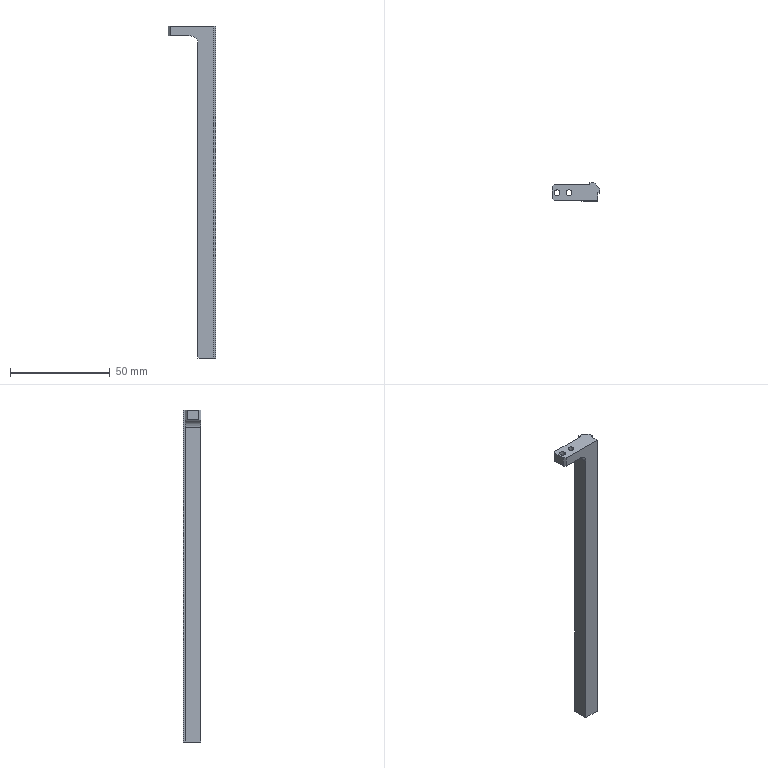NC program | NX | posted with a generic post | part box 24 x 9 x 166.5 mm
Whole program:
N10 G17 G21 G94 G90
(FACE_MILLING , TOOL : FACEMILL_D63)
N12 T01 M6
N14 G54
N16 G17 G0 G90 X-126.45 Y0. S4000 M3
N18 G43 Z20. H1
N20 G94 G1 Z0. F5000.
N22 X-117. F800.
N24 X117.
N26 X126.45
N28 G0 Z20.
N30 M5
(DYNAMIC_ROUGH , TOOL : D8-25-D8-60-3T-ROUGH)
N32 T02 M6
N34 G54
N36 G17 G0 G90 X92.04 Y3.501 S6500 M3
N38 G43 Z20. H2
N40 Z-10.5
N42 G94 G1 X92.015 Y3.499 Z-10.656 F3000.
N44 X91.991 Y3.497 Z-10.718
N46 X91.966 Y3.495 Z-10.763
N48 X91.941 Y3.493 Z-10.8
N50 X91.916 Y3.491 Z-10.831
N52 X91.891 Y3.489 Z-10.857
N54 X91.866 Y3.487 Z-10.88
N56 X91.841 Y3.485 Z-10.9
N58 X91.816 Y3.483 Z-10.918
N60 X91.791 Y3.481 Z-10.933
N62 X91.766 Y3.479 Z-10.947
N64 X91.741 Y3.477 Z-10.958
N66 X91.716 Y3.474 Z-10.968
N68 X91.692 Y3.472 Z-10.977
N70 X91.667 Y3.47 Z-10.984
N72 X91.642 Y3.468 Z-10.99
N74 X91.617 Y3.466 Z-10.994
N76 X91.592 Y3.464 Z-10.997
N78 X91.567 Y3.462 Z-10.999
N80 X91.542 Y3.46 Z-11.
N82 X90.193 Y3.35
N84 G3 X89.546 Y2.925 R0.809
N86 X88.822 Y0.359 R7.041
N88 X88.527 Y-5.709 R56.686
N90 G2 X88.481 Y-10.33 R413.5
N92 X86.629 Y-13.306 R4.525
N94 X82.787 Y-14.912 R9.339
N96 X77.117 Y-15.428 R33.802
N98 X65.718 Y-15.498 R574.286
N100 G1 X-75.866 Y-15.499
N102 G3 X-76.449 Y-15.739 R1.175
N104 G1 X-77.327 Y-16.046
N106 X-78.251 Y-16.15
N108 X-83.251
N110 X-84.173 Y-16.046
N112 X-85.051 Y-15.739
N114 X-85.837 Y-15.245
N116 X-86.495 Y-14.587
N118 G2 X-87.868 Y-11.251 R8.727
N120 X-88.416 Y-5.736 R30.867
N122 X-88.484 Y10.263 R613.548
N124 X-87.442 Y12.546 R4.163
N126 G3 X-87.296 Y12.923 R1.408
N128 G1 X-86.989 Y13.801
N130 X-86.495 Y14.587
N132 X-85.837 Y15.245
N134 X-85.051 Y15.739
N136 X-84.173 Y16.046
N138 X-83.249 Y16.15
N140 X83.251
N142 X84.173 Y16.046
N144 X85.051 Y15.739
N146 X85.837 Y15.245
N148 X86.495 Y14.587
N150 G2 X87.869 Y11.247 R8.729
N152 X88.36 Y4.982 R25.315
N154 G3 X87.818 Y-0.011 R824.39
N156 X87.514 Y-7.66 R117.924
N158 G2 X84.938 Y-12.045 R5.963
N160 X80.581 Y-13.828 R11.133
N162 X74.317 Y-14.417 R37.175
N164 X62.392 Y-14.497 R521.568
N166 G1 X-73.515 Y-14.498
N168 G3 X-74.911 Y-14.604 R5.765
N170 G1 X-75.177 Y-14.76
N172 G2 X-76.234 Y-15.604 R3.529
N174 G3 X-75.071 Y-14.653 R4.07
N176 G2 X-73.492 Y-14.176 R3.891
N178 X-68.214 Y-13.917 R44.777
N180 G1 X-61.946 Y-13.898
N182 X65.154 Y-13.896
N184 G3 X75.877 Y-13.729 R210.065
N186 X81.204 Y-12.923 R23.311
N188 X84.578 Y-11.011 R7.69
N190 X86.383 Y-7.437 R7.723
N192 X86.976 Y-3.056 R28.228
N194 G2 X87.641 Y4.04 R321.595
N196 G3 X87.4 Y9.877 R26.845
N198 G1 Y12.
N200 X87.296 Y12.923
N202 X86.989 Y13.801
N204 X87.296 Y12.923
N206 X87.4 Y12.
N208 Y2.999
N210 X87.296 Y2.077
N212 G3 X86.129 Y-2.669 R18.763
N214 G2 X85.377 Y-6.642 R25.565
N216 X81.646 Y-10.952 R7.379
N218 X76.555 Y-12.443 R15.205
N220 X68.997 Y-12.863 R64.21
N222 G1 X58.572 Y-12.897
N224 X-63.397 Y-12.898
N226 G3 X-71.446 Y-13.05 R128.548
N228 X-74.162 Y-13.532 R10.283
N230 X-74.52 Y-13.814 R1.243
N232 G2 X-75.111 Y-14.694 R4.84
N234 G3 X-74.476 Y-13.734 R4.989
N236 G2 X-73.386 Y-13.065 R2.302
N238 X-69.737 Y-12.458 R14.201
N240 X-61.269 Y-12.298 R147.584
N242 G1 X58.754
N244 G3 X71.903 Y-12.18 R390.996
N246 X78.003 Y-11.477 R31.973
N248 X82.054 Y-9.607 R9.974
N250 X84.616 Y-5.704 R8.61
N252 X85.652 Y-1.59 R35.363
N254 G2 X86.064 Y-0.063 R9.526
N256 X86.495 Y0.413 R2.986
N258 G1 X86.989 Y1.199
N260 X86.495 Y0.413
N262 G3 X85.019 Y-1.762 R5.148
N264 G2 X83.666 Y-5.178 R58.952
N266 X78.794 Y-9.678 R9.039
N268 X73.182 Y-10.954 R19.738
N270 X64.267 Y-11.281 R100.278
N272 G1 X55.417 Y-11.297
N274 X-60.696 Y-11.299
N276 G3 X-69.199 Y-11.472 R136.337
N278 X-73.009 Y-12.139 R14.86
N280 X-74.057 Y-12.703 R2.897
N282 G1 X-74.212 Y-12.945
N284 X-74.511 Y-13.801
N286 X-74.159 Y-12.781
N288 G2 X-72.878 Y-11.816 R2.774
N290 X-69.165 Y-10.98 R12.632
N292 X-61.331 Y-10.707 R88.006
N294 G1 X-56.096 Y-10.697
N296 X59.529 Y-10.695
N298 G3 X70.701 Y-10.513 R218.057
N300 X76.625 Y-9.641 R27.38
N302 X81.401 Y-6.811 R9.957
N304 X83.623 Y-3.265 R14.413
N306 G2 X84.842 Y-0.923 R20.753
N308 G1 X85.07 Y-0.727
N310 G3 X85.944 Y-0.139 R4.796
N312 G2 X84.781 Y-0.86 R4.613
N314 G3 X83.35 Y-2.41 R5.863
N316 G2 X81.221 Y-5.222 R26.449
N318 X75.576 Y-8.542 R12.045
N320 X69.359 Y-9.486 R29.39
N322 X58.412 Y-9.693 R196.812
N324 G1 X53.612 Y-9.697
N326 X-57.697 Y-9.698
N328 G3 X-67.413 Y-9.886 R158.154
N330 X-72.053 Y-10.679 R18.532
N332 X-73.935 Y-11.756 R4.815
N334 X-74.118 Y-12.156 R1.287
N336 G1 X-74.204 Y-12.923
N338 X-74.1 Y-12.001
N340 G2 X-73.215 Y-10.948 R2.12
N342 X-70.062 Y-9.741 R8.553
N344 X-64.019 Y-9.178 R36.636
N346 X-54.671 Y-9.097 R407.332
N348 G1 X56.754 Y-9.095
N350 G3 X68.152 Y-8.93 R254.128
N352 X74.536 Y-8.088 R32.345
N354 X81.433 Y-3.721 R12.634
N356 G2 X83.542 Y-1.329 R28.766
N358 X84.173 Y-1.046 R0.965
N360 G1 X84.952 Y-0.773
N362 G2 X84.029 Y-1.062 R4.368
N364 G3 X82.743 Y-1.58 R2.441
N366 X80.273 Y-3.64 R34.223
N368 G2 X72.75 Y-7.23 R16.232
N370 X65.522 Y-7.975 R43.439
N372 X52.623 Y-8.096 R414.666
N374 G1 X-54.025 Y-8.097
N376 G3 X-65.124 Y-8.251 R236.531
N378 X-70.762 Y-9.036 R26.178
N380 X-73.655 Y-10.5 R7.121
N382 X-74.1 Y-11.249 R1.158
N384 G1 Y-12.001
N386 Y-11.099
N388 G2 X-73.325 Y-9.95 R2.119
N390 X-70.262 Y-8.464 R7.844
N392 X-64.46 Y-7.665 R28.232
N394 X-53.62 Y-7.498 R223.232
N396 G1 X50.579 Y-7.497
N398 G3 X64.928 Y-7.382 R486.963
N400 X72.085 Y-6.672 R44.486
N402 X79.833 Y-3.063 R17.368
N404 G2 X82.394 Y-1.243 R19.765
N406 X83.249 Y-1.15 R1.904
N408 G1 X83.771 Y-1.091
N410 G2 X82.355 Y-1.15 R8.516
N412 G3 X80.216 Y-1.964 R6.073
N414 G2 X76.295 Y-4.076 R52.076
N416 X68.548 Y-6.048 R25.204
N418 X59.336 Y-6.467 R95.672
N420 G1 X48.011 Y-6.497
N422 X-53.423 Y-6.498
N424 G3 X-64.207 Y-6.685 R200.665
N426 X-70.135 Y-7.55 R28.08
N428 X-73.458 Y-9.212 R8.514
N430 X-74.067 Y-9.99 R1.925
N432 X-74.1 Y-11.143 R6.16
N434 G1 X-74.094 Y-9.943
N436 G2 X-73.045 Y-8.552 R2.913
N438 X-69.606 Y-6.946 R9.396
N440 X-63.581 Y-6.096 R30.323
N442 X-52.12 Y-5.898 R213.101
N444 G1 X48.404 Y-5.897
N446 G3 X63.203 Y-5.779 R503.536
N448 X71.032 Y-5.007 R48.745
N450 X77.985 Y-2.452 R24.546
N452 G2 X80.667 Y-1.172 R22.225
N454 X82.386 Y-1.15 R18.999
N456 G3 X79.868 Y-1.177 R32.283
N458 X77.171 Y-1.975 R13.915
N460 G2 X65.488 Y-4.599 R36.687
N462 X54.319 Y-4.887 R169.644
N464 G1 X46.819 Y-4.897
N466 X-51.848 Y-4.898
N468 G3 X-63.225 Y-5.108 R202.281
N470 X-69.609 Y-6.057 R30.448
N472 X-73.246 Y-7.838 R9.799
N474 X-74.053 Y-8.784 R2.728
N476 G1 X-74.1 Y-9.003
N478 Y-10.053
N480 Y-8.853
N482 G2 X-73.254 Y-7.517 R2.642
N484 X-69.927 Y-5.691 R8.827
N486 X-63.838 Y-4.602 R26.701
N488 X-53.984 Y-4.306 R133.89
N490 G1 X-49.346 Y-4.297
N492 X49.629 Y-4.295
N494 G3 X63.127 Y-4.118 R322.68
N496 X71.891 Y-2.989 R45.301
N498 X77.108 Y-1.356 R64.058
N500 G2 X77.842 Y-1.15 R18.45
N502 G1 X80.167
N504 G3 X76.25 Y-1.168 R168.279
N506 X72.386 Y-1.88 R38.541
N508 G2 X60.773 Y-3.172 R63.645
N510 X44.65 Y-3.297 R571.956
N512 G1 X-50.422 Y-3.298
N514 G3 X-62.248 Y-3.524 R206.989
N516 X-69.093 Y-4.54 R33.173
N518 X-73.034 Y-6.415 R11.137
N520 X-74.047 Y-7.547 R3.465
N522 G1 X-74.1 Y-7.783
N524 Y-8.908
N526 Y-7.633
N528 G2 X-73.177 Y-6.184 R2.873
N530 X-69.613 Y-4.223 R9.627
N532 X-63.151 Y-3.036 R28.232
N534 X-53.003 Y-2.71 R131.453
N536 G1 X-45.221 Y-2.697
N538 X47.754 Y-2.695
N540 G3 X61.702 Y-2.522 R360.141
N542 X72.889 Y-1.15 R67.055
N544 G1 X76.564
N546 G3 X67.491 Y-1.167 R617.669
N548 G2 X50.94 Y-1.685 R225.211
N550 G1 X38.49 Y-1.697
N552 X-47.874 Y-1.699
N554 G3 X-60.624 Y-1.898 R264.925
N556 X-68.101 Y-2.877 R39.862
N558 X-72.564 Y-4.769 R13.517
N560 X-74.011 Y-6.2 R5.343
N562 G1 X-74.1 Y-6.525
N564 Y-7.65
N566 Y-6.375
N568 G2 X-73.239 Y-4.951 R2.853
N570 X-69.73 Y-2.886 R9.624
N572 X-63.172 Y-1.533 R27.214
N574 X-55.321 Y-1.15 R96.17
N576 G1 X67.829
N578 X67.964 Y-1.163
N580 X68.096 Y-1.195
N582 X69.068 Y-1.535
N584 G2 X68.802 Y-3.106 R0.808
N586 G1 X68.777 Z-10.999
N588 X68.752 Z-10.997
N590 X68.727 Z-10.994
N592 X68.702 Z-10.99
N594 X68.677 Z-10.984
N596 X68.652 Z-10.977
N598 X68.627 Z-10.968
N600 X68.602 Z-10.958
N602 X68.577 Z-10.947
N604 X68.552 Z-10.933
N606 X68.527 Z-10.918
N608 X68.502 Z-10.9
N610 X68.477 Z-10.88
N612 X68.452 Z-10.857
N614 X68.427 Z-10.831
N616 X68.402 Z-10.8
N618 X68.377 Z-10.763
N620 X68.352 Z-10.718
N622 X68.327 Z-10.656
N624 X68.302 Z-10.5
N626 G0 Z20.
N628 X-53.07
N630 Z-10.5
N632 G1 X-53.095 Z-10.656
N634 X-53.12 Z-10.718
N636 X-53.145 Z-10.763
N638 X-53.17 Z-10.8
N640 X-53.195 Z-10.831
N642 X-53.22 Z-10.857
N644 X-53.245 Z-10.88
N646 X-53.27 Z-10.9
N648 X-53.295 Z-10.918
N650 X-53.32 Z-10.933
N652 X-53.345 Z-10.947
N654 X-53.37 Z-10.958
N656 X-53.395 Z-10.968
N658 X-53.42 Z-10.977
N660 X-53.445 Z-10.984
N662 X-53.47 Z-10.99
N664 X-53.495 Z-10.994
N666 X-53.52 Z-10.997
N668 X-53.545 Z-10.999
N670 X-53.57 Z-11.
N672 G2 X-54.354 Y-2.493 R0.808
N674 G1 X-54.537 Y-1.762
N676 G3 X-55.321 Y-1.15 R0.808
N678 G1 X-65.683 Y-1.165
N680 G3 X-72.089 Y-3.135 R14.586
N682 X-73.992 Y-4.866 R6.277
N684 X-74.1 Y-5.224 R2.837
N686 G1 Y-6.424
N688 Y-5.074
N690 G2 X-73.187 Y-3.589 R3.012
N692 X-69.564 Y-1.491 R9.657
N694 X-68.387 Y-1.15 R13.019
N696 G1 X-65.387
N698 X-69.641 Y-1.16
N700 G3 X-73.974 Y-3.582 R6.322
N702 X-74.1 Y-3.977 R1.533
N704 G1 Y-5.102
N706 Y-3.827
N708 G2 X-73.161 Y-2.356 R2.822
N710 X-71.126 Y-1.157 R5.202
N712 G1 X-69.488 Y-1.15
N714 X-71.724 Y-1.165
N716 G3 X-74.016 Y-2.611 R3.408
N718 G1 X-74.1 Y-2.924
N720 Y-3.899
N722 Y-2.774
N724 G2 X-73.156 Y-1.486 R2.195
N726 X-72.429 Y-1.15 R1.55
N728 G1 X-71.529
N730 G3 X-72.871 Y-1.169 R29.249
N732 X-74.008 Y-1.912 R1.692
N734 G1 X-74.1 Y-2.245
N736 Y-2.845
N738 X-74.093 Y-2.02
N740 G2 X-73.128 Y-1.15 R1.19
N742 G1 X-72.678
N744 X-73.429 Y-1.172
N746 G3 X-74.1 Y-2.162 R0.89
N748 X-73.737 Y-2.833 R0.801
N750 G1 X-73.458 Y-3.014
N752 X-72.147 Y-3.869 Z-10.9
N754 G2 X-71.78 Y-4.16 R1.373 F15000.
N756 X-71.611 Y-4.652 R0.808
N758 G1 Y-11.986
N760 G2 X-72.155 Y-14.815 R7.625
N762 G1 X-72.298 Y-15.169
N764 X-72.449 Y-15.52
N766 G2 X-73.493 Y-16.742 R3.323
N768 X-75.768 Y-18.159 R22.76
N770 X-77.409 Y-18.578 R4.415
N772 G1 X-83.488 Y-18.972
N774 G2 X-85.925 Y-18.191 R3.495
N776 G1 X-86.989 Y-17.321
N778 G2 X-87.275 Y-16.592 R0.801
N780 G1 X-87.068 Y-15.042 Z-11. F3000.
N782 X-86.951 Y-14.171
N784 G3 X-86.989 Y-13.801 R0.843
N786 G1 X-87.296 Y-12.923
N788 X-87.4 Y-11.999
N790 Y12.001
N792 X-87.299 Y12.895
N794 G3 X-87.714 Y13.694 R0.809
N796 G1 X-88.876 Y14.331
N798 X-88.898 Y14.343 Z-10.999
N800 X-88.92 Y14.355 Z-10.997
N802 X-88.941 Y14.367 Z-10.994
N804 X-88.963 Y14.379 Z-10.99
N806 X-88.985 Y14.391 Z-10.984
N808 X-89.007 Y14.403 Z-10.977
N810 X-89.029 Y14.415 Z-10.968
N812 X-89.051 Y14.427 Z-10.958
N814 X-89.073 Y14.439 Z-10.947
N816 X-89.095 Y14.451 Z-10.933
N818 X-89.117 Y14.463 Z-10.918
N820 X-89.139 Y14.475 Z-10.9
N822 X-89.161 Y14.487 Z-10.88
N824 X-89.183 Y14.499 Z-10.857
N826 X-89.205 Y14.511 Z-10.831
N828 X-89.227 Y14.523 Z-10.8
N830 X-89.248 Y14.535 Z-10.763
N832 X-89.27 Y14.547 Z-10.718
N834 X-89.292 Y14.559 Z-10.656
N836 X-89.314 Y14.571 Z-10.5
N838 G0 Z20.
N840 M5
(PLANAR_MILL_COPY_1_COPY_COPY , TOOL : D8R0-FINISH)
N842 T03 M6
N844 G54
N846 G17 G0 G90 X88.25 Y4. S6500 M3
N848 G43 Z20. H3
N850 G94 G1 Z-11. F5000.
N852 G3 X87.25 Y3. R1. F500.
N854 G2 X83.25 Y-1. R4.
N856 G1 X-65.45
N858 X-74.25 F250.
N860 G2 X-74.15 Y-1.889 R4.
N862 G1 Y-5.393
N864 Y-12. F500.
N866 G2 X-78.15 Y-16. R4.
N868 G1 X-83.25
N870 G2 X-87.25 Y-12. R4.
N872 G1 Y12.
N874 G2 X-83.25 Y16. R4.
N876 G1 X83.25
N878 G2 X87.25 Y12. R4.
N880 G1 Y3.
N882 G3 X88.25 Y2. R1.
N884 G1 Y4.
N886 G3 X87.25 Y3. R1.
N888 G2 X83.25 Y-1. R4.
N890 G1 X-65.45
N892 X-74.25 F250.
N894 G2 X-74.15 Y-1.889 R4.
N896 G1 Y-5.393
N898 Y-12. F500.
N900 G2 X-78.15 Y-16. R4.
N902 G1 X-83.25
N904 G2 X-87.25 Y-12. R4.
N906 G1 Y12.
N908 G2 X-83.25 Y16. R4.
N910 G1 X83.25
N912 G2 X87.25 Y12. R4.
N914 G1 Y3.
N916 G3 X88.25 Y2. R1.
N918 G0 Z20.
N920 M5
(PLANAR_MILL_2 , TOOL : DJ-D3)
N922 T08 M6
N924 G54
N926 G17 G0 G90 X87.063 Y1.826 S3500 M3
N928 G43 Z20. H8
N930 Z1.
N932 G94 G1 Z-1. F1000.
N934 G41 X86.078 Y2. D8
N936 X83.249
N938 X-74.25
N940 G3 X-77.175 Y-1.667 R3.
N942 G2 X-77.15 Y-1.889 R1.
N944 G1 Y-12.
N946 G2 X-78.15 Y-13. R1.
N948 G1 X-83.25
N950 G2 X-84.25 Y-12. R1.
N952 G1 Y12.
N954 G2 X-83.25 Y13. R1.
N956 G1 X83.25
N958 G2 X84.25 Y12. R1.
N960 G1 Y3.001
N962 Y0.172
N964 G40
N966 X84.424 Y-0.813
N968 Z1.
N970 G0 Z20.
(PLANAR_MILL_2_COPY , TOOL : DJ-D3)
N972 X-74.065 Y-12.474
N974 Z0.8
N976 G1 Z-1.2 F600.
N978 G41 X-75.05 Y-12.3
N980 X-78.25
N982 X-83.25
N984 X-86.45
N986 G40
N988 X-87.435 Y-12.474
N990 Z0.8
N992 G0 Z20.
(PLANAR_MILL_2_COPY_COPY , TOOL : DJ-D3)
N994 X-74.065 Y-12.374
N996 Z0.8
N998 G1 Z-1.2
N1000 G41 X-75.05 Y-12.2
N1002 X-78.25
N1004 X-83.25
N1006 X-86.45
N1008 G40
N1010 X-87.435 Y-12.374
N1012 Z0.8
N1014 G0 Z20.
N1016 M5
(DRILLING_2 , TOOL : DJ-D8)
N1018 T04 M6
N1020 G54
N1022 G17 G0 G90 X-8.5 Y4. S2000 M3
N1024 G43 Z20. H4
N1026 G94 G81 G99 Z-1.5 F200. R3.
N1028 X-2.5
N1030 G80
N1032 G0 X-2.5 Y4. Z20.
N1034 M5
(DRILLING_2_COPY , TOOL : DRILL_D2.9-39-67)
N1036 T08 M6
N1038 G54
N1040 G17 G0 G90 X-8.5 Y4. S2500 M3
N1042 G43 Z20. H8
N1044 G94 G81 G99 Z-7. F200. R3.
N1046 X-2.5
N1048 G80
N1050 G0 X-2.5 Y4. Z20.
N1052 M5
(DRILLING_3 , TOOL : DJ-D3)
N1054 M6
N1056 G54
N1058 G17 G0 G90 X-5.03 Y-2.97 S2000 M3
N1060 G43 Z20. H8
N1062 G94 G81 G99 Z-1. F200. R3.
N1064 X-1.84 Y-6.16
N1066 G80
N1068 G0 X-1.84 Y-6.16 Z20.
N1070 M5
(DRILLING_3_COPY , TOOL : D1.8_DRILL)
N1072 T06 M6
N1074 G54
N1076 G17 G0 G90 X-1.84 Y-6.16 S2000 M3
N1078 G43 Z20. H6
N1080 G94 G83 G99 Z-8. F200. Q1.5 R3.
N1082 X-5.03 Y-2.97
N1084 G80
N1086 G0 X-5.03 Y-2.97 Z20.
N1088 M5
(FACE_MILLING_COPY , TOOL : D50)
N1090 T01 M6
N1092 G54
N1094 G17 G0 G90 X0. Y115.75 S4000 M3
N1096 G43 Z26. H1
N1098 G94 G1 Z5.025 F5000.
N1100 Y108.25 F1500.
N1102 Y-108.25
N1104 Y-115.75
N1106 G0 Z16.
N1108 Y115.75
N1110 G1 Z4.05 F5000.
N1112 Y108.25 F1500.
N1114 Y-108.25
N1116 Y-115.75
N1118 G0 Z16.
N1120 Y115.75
N1122 G1 Z3.075 F5000.
N1124 Y108.25 F1500.
N1126 Y-108.25
N1128 Y-115.75
N1130 G0 Z16.
N1132 Y115.75
N1134 G1 Z2.1 F5000.
N1136 Y108.25 F1500.
N1138 Y-108.25
N1140 Y-115.75
N1142 G0 Z16.
N1144 Y115.75
N1146 G1 Z1.125 F5000.
N1148 Y108.25 F1500.
N1150 Y-108.25
N1152 Y-115.75
N1154 G0 Z16.
N1156 Y115.75
N1158 G1 Z0.15 F5000.
N1160 Y108.25 F1500.
N1162 Y-108.25
N1164 Y-115.75
N1166 G0 Z26.
(FACE_MILLING_COPY_COPY , TOOL : D50)
N1168 Y115.75
N1170 G1 Z0. F5000.
N1172 Y108.25 F800.
N1174 Y-108.25
N1176 Y-115.75
N1178 G0 Z26.
(PLANAR_MILL , TOOL : D50)
N1180 X18.5 Y133.25
N1182 Z20.
N1184 Z2.1
N1186 G1 Z-0.9 F600.
N1188 Y83.25
N1190 Y-83.25
N1192 Y-133.25
N1194 Z2.1
N1196 G0 Z20.
N1198 M5
(PLANAR_MILL_COPY_2 , TOOL : D8-25-D8-60-3T-FINISH)
N1200 T03 M6
N1202 G54
N1204 G17 G0 G90 X-0.6 Y72.25 S5500 M3
N1206 G43 Z19. H3
N1208 G94 G1 Z-1. F5000.
N1210 Y78.25 F1500.
N1212 Y83.25
N1214 Y89.25
N1216 G0 Z4.
N1218 X4.2 Y72.25
N1220 G1 Z-1. F5000.
N1222 Y78.25 F1500.
N1224 Y83.25
N1226 Y89.25
N1228 G0 Z4.
N1230 X9. Y72.25
N1232 G1 Z-1. F5000.
N1234 Y78.25 F1500.
N1236 Y83.25
N1238 Y89.25
N1240 G0 Z19.
(PLANAR_MILL_COPY_2_COPY , TOOL : D8-25-D8-60-3T-FINISH)
N1242 Z20.
N1244 X-2.9 Y89.25
N1246 G1 Z-0.9 F5000.
N1248 Y83.25 F1500.
N1250 Y-83.25
N1252 Y-89.25
N1254 G0 Z20.
(PLANAR_MILL_COPY_2_COPY_COPY , TOOL : D8-25-D8-60-3T-FINISH)
N1256 X-3. Y89.25
N1258 G1 Z-1. F5000.
N1260 Y83.25 F800.
N1262 Y-83.25
N1264 Y-89.25
N1266 G0 Z20.
N1268 M5
(DRILLING , TOOL : DJ-D3)
N1270 T04 M6
N1272 G54
N1274 G17 G0 G90 X-4.5 Y24. S2000 M3
N1276 G43 Z29. H4
N1278 G94 G81 G99 Z-2.1 F200. R0.
N1280 G0 Z29.
N1282 G81 Y-36. Z-2.1 R0.
N1284 G0 Z29.
N1286 G80
N1288 G0 X-4.5 Y-36. Z29.
(PLANAR_MILL_COPY_2_COPY_1_COPY_1 , TOOL : DJ-D3)
N1290 X-14.75 Y83.15 S5000
N1292 Z20.
N1294 G1 Z-0.6 F5000.
N1296 G41 X-12.5 F1000. D4
N1298 G2 X-11.9 Y83.75 R0.6
N1300 G1 X-7.1
N1302 G2 X-6.5 Y83.15 R0.6
N1304 G1 Y-83.15
N1306 G2 X-7.1 Y-83.75 R0.6
N1308 G1 X-11.9
N1310 G2 X-12.5 Y-83.15 R0.6
N1312 G1 Y83.15
N1314 G40
N1316 X-14.75
N1318 G0 Z20.
(PLANAR_MILL_COPY_2_COPY_1_COPY_1_COPY , TOOL : DJ-D3)
N1320 X-5.997 Y85.35
N1322 Z19.
N1324 G1 Z0. F5000.
N1326 Z-2. F1000.
N1328 G41 X-6. Y85.15
N1330 G3 X-5. Y84.15 R1.
N1332 G1 X11.9
N1334 G2 X12.9 Y83.15 R1.
N1336 G1 Y78.35
N1338 G2 X11.9 Y77.35 R1.
N1340 G1 X11.336
N1342 G2 X10.9 Y77.25 R1.
N1344 G1 X0.219
N1346 G3 X-2.1 Y74.25 R3.1
N1348 G1 Y-83.25
N1350 Y-84.75
N1352 G40
N1354 X-2.097 Y-84.95
N1356 G0 Z19.
(PLANAR_MILL_COPY_2_COPY_1_COPY_1_COPY_COPY , TOOL : DJ-D3)
N1358 X12.303 Y85.65
N1360 G1 Z-0.2 F5000.
N1362 Z-2.2 F600.
N1364 G41 X12.3 Y83.25
N1366 Y78.25
N1368 Y76.05
N1370 G40
N1372 X12.303 Y75.85
N1374 Z-0.2
N1376 G0 Z19.
(PLANAR_MILL_COPY_2_COPY_1_COPY_1_COPY_COPY_COPY , TOOL : DJ-D3)
N1378 X12.203 Y85.65
N1380 G1 Z-0.2 F5000.
N1382 Z-2.2 F600.
N1384 G41 X12.2 Y83.25
N1386 Y78.25
N1388 Y76.05
N1390 G40
N1392 X12.203 Y75.85
N1394 Z-0.2
N1396 G0 Z19.
N1398 M5
(DRILLING_COPY , TOOL : D1.8_DRILL)
N1400 T06 M6
N1402 G54
N1404 G17 G0 G90 X-4.5 Y24. S2000 M3
N1406 G43 Z29. H6
N1408 G94 G81 G99 Z-7.5 F100. R0.
N1410 G0 Z29.
N1412 G81 Y-36. Z-7.5 R0.
N1414 G0 Z29.
N1416 G80
N1418 G0 X-4.5 Y-36. Z29.
N1420 M5
(PLANAR_MILL_3 , TOOL : DJ-D3)
N1422 T00 M6
N1424 G54
N1426 G17 G0 G90 X-8.3 Y-7.8 S4500 M3
N1428 G43 Z20. H0
N1430 Z1.7
N1432 G94 G1 Z-1.3 F800.
N1434 Y-5.
N1436 Y0.
N1438 Y2.8
N1440 Z1.7
N1442 G0 Z20.
N1444 X0.3
N1446 Z1.7
N1448 G1 Z-1.3
N1450 Y0.
N1452 Y-5.
N1454 Y-7.8
N1456 Z1.7
N1458 G0 Z20.
(DRILLING_1 , TOOL : DJ-D3)
N1460 X-1.5 Y-115.25 S2500
N1462 G81 G99 Z-16.1 F200. R-12.
N1464 G80
N1466 G0 X-1.5 Y-115.25 Z20.
N1468 M5
(DRILLING_1_COPY , TOOL : DRILL_D2.3-29-55)
N1470 M6
N1472 G54
N1474 G17 G0 G90 X-1.5 Y-115.25 S2500 M3
N1476 G43 Z20. H0
N1478 G94 G81 G99 Z-22. F200. R-12.
N1480 G80
N1482 G0 X-1.5 Y-115.25 Z20.
N1484 M5
(DRILLING_1_COPY_COPY , TOOL : FORMTAP_M2.5-12-D3-39)
N1486 M6
N1488 G54
N1490 G17 G0 G90 X-1.5 Y-115.25 S300 M3
N1492 G43 Z20. H0
N1494 G84 G94 G99 Z-21. F135. R-12.
N1496 G80
N1498 G0 X-1.5 Y-115.25 Z20.
N1500 M5
(PLANAR_MILL_COPY_2_COPY_1_COPY_1_COPY_1 , TOOL : D8-25-D8-60-3T-ROUGH)
N1502 T02 M6
N1504 G54
N1506 G17 G0 G90 X-0.1 Y-172.5 S5000 M3
N1508 G43 Z21. H2
N1510 G94 G1 Z0.1 F5000.
N1512 Y-166.5 F1200.
N1514 Y0.
N1516 Y6.
N1518 G0 Z21.
(ZLEVEL_PROFILE , TOOL : D8-25-D8-60-3T-ROUGH)
N1520 X10.712 Y5.2
N1522 G1 Z0.5 F5000.
N1524 Y0. F3000.
N1526 Y-166.5
N1528 Y-171.7
N1530 G0 X11.212 Z0.
N1532 G1 Y-166.5
N1534 Y0.
N1536 Y5.2
N1538 G0 X11.712 Z-0.5
N1540 G1 Y0.
N1542 Y-166.5
N1544 Y-171.7
N1546 G0 X12.212 Z-1.
N1548 G1 Y-166.5
N1550 Y0.
N1552 Y5.2
N1554 G0 X12.712 Z-1.5
N1556 G1 Y0.
N1558 Y-166.5
N1560 Y-171.7
N1562 G0 Z21.
N1564 M5
(PLANAR_MILL_COPY_2_COPY_1_COPY_1_COPY_1_COPY_2 , TOOL : D8R0-FINISH)
N1566 T03 M6
N1568 G54
N1570 G17 G0 G90 X0. Y-172.5 S5000 M3
N1572 G43 Z21. H3
N1574 G94 G1 Z0. F5000.
N1576 Y-166.5 F1200.
N1578 Y0.
N1580 Y6.
N1582 G0 Z21.
N1584 M5
(PLANAR_MILL_COPY_2_COPY_1_COPY_1_COPY_1_COPY_COPY , TOOL : DJ-D8)
N1586 T08 M6
N1588 G54
N1590 G17 G0 G90 X9.509 Y6.5 S5000 M3
N1592 G43 Z21. H8
N1594 G94 G1 Z-2.5 F5000.
N1596 G41 X9.5 Y6. F800. D8
N1598 Y0.
N1600 Y-166.5
N1602 Y-172.5
N1604 G40
N1606 X9.509 Y-173.
N1608 G0 Z21.
N1610 M5
(DRILLING_COPY_1 , TOOL : DJ-D3)
N1612 T04 M6
N1614 G54
N1616 G17 G0 G90 X1.5 Y-143.25 S2000 M3
N1618 G43 Z30. H4
N1620 G94 G81 G99 Z-1.1 F200. R1.
N1622 G0 Z30.
N1624 G81 Y-78.25 Z-1.1 R1.
N1626 G0 Z30.
N1628 G81 Y-13.25 Z-1.1 R1.
N1630 G0 Z30.
N1632 G80
N1634 G0 X1.5 Y-13.25 Z30.
(PLANAR_MILL_COPY_2_COPY_1_COPY_1_COPY_1_COPY_COPY_COPY , TOOL : DJ-D3)
N1636 X8.75 Y-167.209 S5000
N1638 Z21.
N1640 G1 Z0.2 F5000.
N1642 G41 X8.25 Y-167.2 F1000. D4
N1644 X6.
N1646 X4.1
N1648 G2 X3.3 Y-166.4 R0.8
N1650 G1 Y-0.1
N1652 G2 X4.1 Y0.7 R0.8
N1654 G1 X6.
N1656 X8.25
N1658 G40
N1660 X8.75 Y0.709
N1662 G0 Z21.
(PLANAR_MILL_COPY_2_COPY_1_COPY_1_COPY_1_COPY_COPY_COPY_COPY , TOOL : DJ-D3)
N1664 X-0.909 Y-169.25
N1666 G1 Z-1. F5000.
N1668 G41 X-0.9 Y-168.75 F1000.
N1670 Y-166.5
N1672 Y0.
N1674 Y2.25
N1676 G40
N1678 X-0.909 Y2.75
N1680 G0 Z21.
N1682 M5
(DRILLING_COPY_COPY_1 , TOOL : D1.8_DRILL)
N1684 T06 M6
N1686 G54
N1688 G17 G0 G90 X1.5 Y-143.25 S2000 M3
N1690 G43 Z30. H6
N1692 G94 G81 G99 Z-6.5 F100. R1.
N1694 G0 Z30.
N1696 G81 Y-78.25 Z-6.5 R1.
N1698 G0 Z30.
N1700 G81 Y-13.25 Z-6.5 R1.
N1702 G0 Z30.
N1704 G80
N1706 G0 X1.5 Y-13.25 Z30.
N1708 M5
N1710 M2